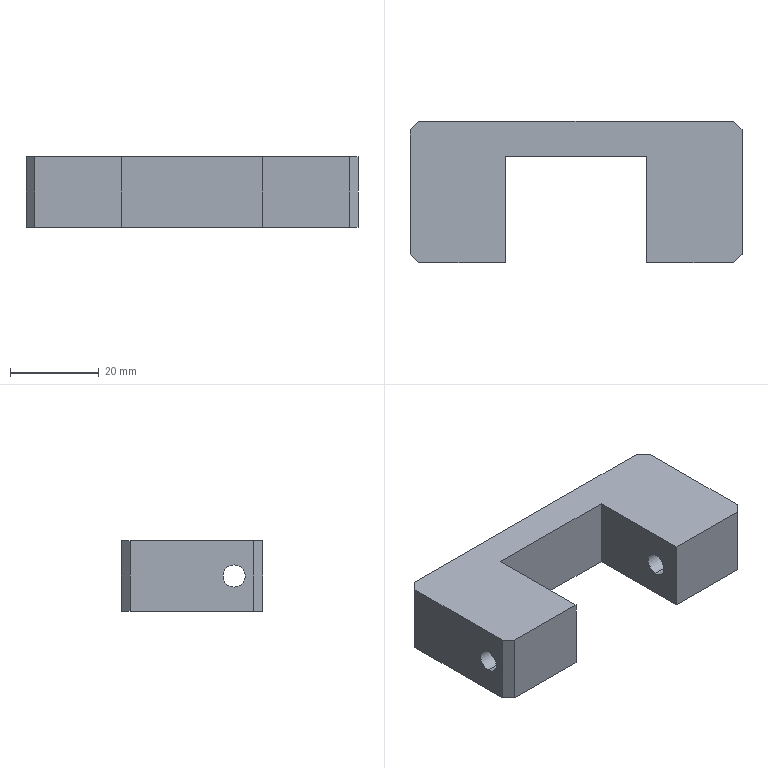Part | SolidWorks | features Chamfer 2, HoleWzd 2, Extrusion 1, ICE 1 | 1 solid | 26 faces | box 75 x 32 x 16 mm | volume 23656 mm3 | plane 14 | cylinder 8 | cone 4 | commonest cylinder face diameters 5 x4 6.8 x4
STEP:
#1=CARTESIAN_POINT('',(-27.5,-3.75,-3.4));
#2=VERTEX_POINT('',#1);
#3=CARTESIAN_POINT('',(-27.5,-3.75,3.4));
#4=VERTEX_POINT('',#3);
#5=CARTESIAN_POINT('',(-27.5,-3.75,0.));
#6=DIRECTION('',(0.,1.,0.));
#7=DIRECTION('',(0.,0.,1.));
#8=AXIS2_PLACEMENT_3D('',#5,#6,#7);
#9=CIRCLE('',#8,3.4);
#10=EDGE_CURVE('',#2,#4,#9,.T.);
#11=ORIENTED_EDGE('',*,*,#10,.F.);
#12=CARTESIAN_POINT('',(-27.5,16.,-3.4));
#13=VERTEX_POINT('',#12);
#14=CARTESIAN_POINT('',(-27.5,16.,-3.4));
#15=DIRECTION('',(0.,1.,0.));
#16=VECTOR('',#15,1000.);
#17=LINE('',#14,#16);
#18=EDGE_CURVE('',#2,#13,#17,.T.);
#19=ORIENTED_EDGE('',*,*,#18,.T.);
#20=CARTESIAN_POINT('',(-27.5,16.,3.4));
#21=VERTEX_POINT('',#20);
#22=CARTESIAN_POINT('',(-27.5,16.,0.));
#23=DIRECTION('',(0.,1.,0.));
#24=DIRECTION('',(0.,0.,1.));
#25=AXIS2_PLACEMENT_3D('',#22,#23,#24);
#26=CIRCLE('',#25,3.4);
#27=EDGE_CURVE('',#13,#21,#26,.T.);
#28=ORIENTED_EDGE('',*,*,#27,.T.);
#29=CARTESIAN_POINT('',(-27.5,16.,3.4));
#30=DIRECTION('',(0.,1.,0.));
#31=VECTOR('',#30,1000.);
#32=LINE('',#29,#31);
#33=EDGE_CURVE('',#4,#21,#32,.T.);
#34=ORIENTED_EDGE('',*,*,#33,.F.);
#35=EDGE_LOOP('',(#11,#19,#28,#34));
#36=FACE_OUTER_BOUND('',#35,.T.);
#37=CARTESIAN_POINT('',(-27.5,16.,0.));
#38=DIRECTION('',(0.,1.,0.));
#39=DIRECTION('',(0.,0.,1.));
#40=AXIS2_PLACEMENT_3D('',#37,#38,#39);
#41=CYLINDRICAL_SURFACE('',#40,3.4);
#42=ADVANCED_FACE('',(#36),#41,.F.);
#43=CARTESIAN_POINT('',(-27.5,-5.793,0.));
#44=VERTEX_POINT('',#43);
#45=CARTESIAN_POINT('',(-27.5,-3.75,3.4));
#46=DIRECTION('',(0.,0.515,0.8572));
#47=VECTOR('',#46,1000.);
#48=LINE('',#45,#47);
#49=EDGE_CURVE('',#44,#4,#48,.T.);
#50=ORIENTED_EDGE('',*,*,#49,.F.);
#51=CARTESIAN_POINT('',(-27.5,-3.75,-3.4));
#52=DIRECTION('',(0.,0.515,-0.8572));
#53=VECTOR('',#52,1000.);
#54=LINE('',#51,#53);
#55=EDGE_CURVE('',#44,#2,#54,.T.);
#56=ORIENTED_EDGE('',*,*,#55,.T.);
#57=ORIENTED_EDGE('',*,*,#10,.T.);
#58=EDGE_LOOP('',(#50,#56,#57));
#59=FACE_OUTER_BOUND('',#58,.T.);
#60=CARTESIAN_POINT('',(-27.5,-3.75,0.));
#61=DIRECTION('',(0.,1.,0.));
#62=DIRECTION('',(0.,0.,1.));
#63=AXIS2_PLACEMENT_3D('',#60,#61,#62);
#64=CONICAL_SURFACE('',#63,3.4,1.03);
#65=ADVANCED_FACE('',(#59),#64,.F.);
#66=CARTESIAN_POINT('',(27.5,-3.75,-3.4));
#67=VERTEX_POINT('',#66);
#68=CARTESIAN_POINT('',(27.5,-3.75,3.4));
#69=VERTEX_POINT('',#68);
#70=CARTESIAN_POINT('',(27.5,-3.75,0.));
#71=DIRECTION('',(0.,1.,0.));
#72=DIRECTION('',(0.,0.,1.));
#73=AXIS2_PLACEMENT_3D('',#70,#71,#72);
#74=CIRCLE('',#73,3.4);
#75=EDGE_CURVE('',#67,#69,#74,.T.);
#76=ORIENTED_EDGE('',*,*,#75,.F.);
#77=CARTESIAN_POINT('',(27.5,16.,-3.4));
#78=VERTEX_POINT('',#77);
#79=CARTESIAN_POINT('',(27.5,16.,-3.4));
#80=DIRECTION('',(0.,1.,0.));
#81=VECTOR('',#80,1000.);
#82=LINE('',#79,#81);
#83=EDGE_CURVE('',#67,#78,#82,.T.);
#84=ORIENTED_EDGE('',*,*,#83,.T.);
#85=CARTESIAN_POINT('',(27.5,16.,3.4));
#86=VERTEX_POINT('',#85);
#87=CARTESIAN_POINT('',(27.5,16.,0.));
#88=DIRECTION('',(0.,1.,0.));
#89=DIRECTION('',(0.,0.,1.));
#90=AXIS2_PLACEMENT_3D('',#87,#88,#89);
#91=CIRCLE('',#90,3.4);
#92=EDGE_CURVE('',#78,#86,#91,.T.);
#93=ORIENTED_EDGE('',*,*,#92,.T.);
#94=CARTESIAN_POINT('',(27.5,16.,3.4));
#95=DIRECTION('',(0.,1.,0.));
#96=VECTOR('',#95,1000.);
#97=LINE('',#94,#96);
#98=EDGE_CURVE('',#69,#86,#97,.T.);
#99=ORIENTED_EDGE('',*,*,#98,.F.);
#100=EDGE_LOOP('',(#76,#84,#93,#99));
#101=FACE_OUTER_BOUND('',#100,.T.);
#102=CARTESIAN_POINT('',(27.5,16.,0.));
#103=DIRECTION('',(0.,1.,0.));
#104=DIRECTION('',(0.,0.,1.));
#105=AXIS2_PLACEMENT_3D('',#102,#103,#104);
#106=CYLINDRICAL_SURFACE('',#105,3.4);
#107=ADVANCED_FACE('',(#101),#106,.F.);
#108=CARTESIAN_POINT('',(27.5,-5.793,0.));
#109=VERTEX_POINT('',#108);
#110=CARTESIAN_POINT('',(27.5,-3.75,3.4));
#111=DIRECTION('',(0.,0.515,0.8572));
#112=VECTOR('',#111,1000.);
#113=LINE('',#110,#112);
#114=EDGE_CURVE('',#109,#69,#113,.T.);
#115=ORIENTED_EDGE('',*,*,#114,.F.);
#116=CARTESIAN_POINT('',(27.5,-3.75,-3.4));
#117=DIRECTION('',(0.,0.515,-0.8572));
#118=VECTOR('',#117,1000.);
#119=LINE('',#116,#118);
#120=EDGE_CURVE('',#109,#67,#119,.T.);
#121=ORIENTED_EDGE('',*,*,#120,.T.);
#122=ORIENTED_EDGE('',*,*,#75,.T.);
#123=EDGE_LOOP('',(#115,#121,#122));
#124=FACE_OUTER_BOUND('',#123,.T.);
#125=CARTESIAN_POINT('',(27.5,-3.75,0.));
#126=DIRECTION('',(0.,1.,0.));
#127=DIRECTION('',(0.,0.,1.));
#128=AXIS2_PLACEMENT_3D('',#125,#126,#127);
#129=CONICAL_SURFACE('',#128,3.4,1.03);
#130=ADVANCED_FACE('',(#124),#129,.F.);
#131=CARTESIAN_POINT('',(-37.5,-9.5,2.5));
#132=VERTEX_POINT('',#131);
#133=CARTESIAN_POINT('',(-37.5,-9.5,-2.5));
#134=VERTEX_POINT('',#133);
#135=CARTESIAN_POINT('',(-37.5,-9.5,0.));
#136=DIRECTION('',(1.,0.,0.));
#137=DIRECTION('',(0.,0.,-1.));
#138=AXIS2_PLACEMENT_3D('',#135,#136,#137);
#139=CIRCLE('',#138,2.5);
#140=EDGE_CURVE('',#132,#134,#139,.T.);
#141=ORIENTED_EDGE('',*,*,#140,.F.);
#142=CARTESIAN_POINT('',(-16.,-9.5,2.5));
#143=VERTEX_POINT('',#142);
#144=CARTESIAN_POINT('',(37.5,-9.5,2.5));
#145=DIRECTION('',(1.,0.,0.));
#146=VECTOR('',#145,1000.);
#147=LINE('',#144,#146);
#148=EDGE_CURVE('',#132,#143,#147,.T.);
#149=ORIENTED_EDGE('',*,*,#148,.T.);
#150=CARTESIAN_POINT('',(-16.,-9.5,-2.5));
#151=VERTEX_POINT('',#150);
#152=CARTESIAN_POINT('',(-16.,-9.5,0.));
#153=DIRECTION('',(-1.,0.,0.));
#154=DIRECTION('',(0.,0.,1.));
#155=AXIS2_PLACEMENT_3D('',#152,#153,#154);
#156=CIRCLE('',#155,2.5);
#157=EDGE_CURVE('',#151,#143,#156,.T.);
#158=ORIENTED_EDGE('',*,*,#157,.F.);
#159=CARTESIAN_POINT('',(37.5,-9.5,-2.5));
#160=DIRECTION('',(1.,0.,0.));
#161=VECTOR('',#160,1000.);
#162=LINE('',#159,#161);
#163=EDGE_CURVE('',#134,#151,#162,.T.);
#164=ORIENTED_EDGE('',*,*,#163,.F.);
#165=EDGE_LOOP('',(#141,#149,#158,#164));
#166=FACE_OUTER_BOUND('',#165,.T.);
#167=CARTESIAN_POINT('',(37.5,-9.5,0.));
#168=DIRECTION('',(1.,0.,0.));
#169=DIRECTION('',(0.,0.,-1.));
#170=AXIS2_PLACEMENT_3D('',#167,#168,#169);
#171=CYLINDRICAL_SURFACE('',#170,2.5);
#172=ADVANCED_FACE('',(#166),#171,.F.);
#173=CARTESIAN_POINT('',(16.,-9.5,2.5));
#174=VERTEX_POINT('',#173);
#175=CARTESIAN_POINT('',(16.,-9.5,-2.5));
#176=VERTEX_POINT('',#175);
#177=CARTESIAN_POINT('',(16.,-9.5,0.));
#178=DIRECTION('',(1.,0.,0.));
#179=DIRECTION('',(0.,1.,0.));
#180=AXIS2_PLACEMENT_3D('',#177,#178,#179);
#181=CIRCLE('',#180,2.5);
#182=EDGE_CURVE('',#174,#176,#181,.T.);
#183=ORIENTED_EDGE('',*,*,#182,.F.);
#184=CARTESIAN_POINT('',(37.5,-9.5,2.5));
#185=VERTEX_POINT('',#184);
#186=CARTESIAN_POINT('',(37.5,-9.5,2.5));
#187=DIRECTION('',(1.,0.,0.));
#188=VECTOR('',#187,1000.);
#189=LINE('',#186,#188);
#190=EDGE_CURVE('',#174,#185,#189,.T.);
#191=ORIENTED_EDGE('',*,*,#190,.T.);
#192=CARTESIAN_POINT('',(37.5,-9.5,-2.5));
#193=VERTEX_POINT('',#192);
#194=CARTESIAN_POINT('',(37.5,-9.5,0.));
#195=DIRECTION('',(1.,0.,0.));
#196=DIRECTION('',(0.,0.,-1.));
#197=AXIS2_PLACEMENT_3D('',#194,#195,#196);
#198=CIRCLE('',#197,2.5);
#199=EDGE_CURVE('',#185,#193,#198,.T.);
#200=ORIENTED_EDGE('',*,*,#199,.T.);
#201=CARTESIAN_POINT('',(37.5,-9.5,-2.5));
#202=DIRECTION('',(1.,0.,0.));
#203=VECTOR('',#202,1000.);
#204=LINE('',#201,#203);
#205=EDGE_CURVE('',#176,#193,#204,.T.);
#206=ORIENTED_EDGE('',*,*,#205,.F.);
#207=EDGE_LOOP('',(#183,#191,#200,#206));
#208=FACE_OUTER_BOUND('',#207,.T.);
#209=CARTESIAN_POINT('',(37.5,-9.5,0.));
#210=DIRECTION('',(1.,0.,0.));
#211=DIRECTION('',(0.,0.,-1.));
#212=AXIS2_PLACEMENT_3D('',#209,#210,#211);
#213=CYLINDRICAL_SURFACE('',#212,2.5);
#214=ADVANCED_FACE('',(#208),#213,.F.);
#215=CARTESIAN_POINT('',(-35.5,-16.,8.));
#216=VERTEX_POINT('',#215);
#217=CARTESIAN_POINT('',(-16.,-16.,8.));
#218=VERTEX_POINT('',#217);
#219=CARTESIAN_POINT('',(-37.5,-16.,8.));
#220=DIRECTION('',(1.,0.,0.));
#221=VECTOR('',#220,1000.);
#222=LINE('',#219,#221);
#223=EDGE_CURVE('',#216,#218,#222,.T.);
#224=ORIENTED_EDGE('',*,*,#223,.F.);
#225=CARTESIAN_POINT('',(-35.5,-16.,-8.));
#226=VERTEX_POINT('',#225);
#227=CARTESIAN_POINT('',(-35.5,-16.,8.));
#228=DIRECTION('',(0.,0.,-1.));
#229=VECTOR('',#228,1000.);
#230=LINE('',#227,#229);
#231=EDGE_CURVE('',#216,#226,#230,.T.);
#232=ORIENTED_EDGE('',*,*,#231,.T.);
#233=CARTESIAN_POINT('',(-16.,-16.,-8.));
#234=VERTEX_POINT('',#233);
#235=CARTESIAN_POINT('',(-37.5,-16.,-8.));
#236=DIRECTION('',(1.,0.,0.));
#237=VECTOR('',#236,1000.);
#238=LINE('',#235,#237);
#239=EDGE_CURVE('',#226,#234,#238,.T.);
#240=ORIENTED_EDGE('',*,*,#239,.T.);
#241=CARTESIAN_POINT('',(-16.,-16.,-8.));
#242=DIRECTION('',(0.,0.,1.));
#243=VECTOR('',#242,1000.);
#244=LINE('',#241,#243);
#245=EDGE_CURVE('',#234,#218,#244,.T.);
#246=ORIENTED_EDGE('',*,*,#245,.T.);
#247=EDGE_LOOP('',(#224,#232,#240,#246));
#248=FACE_OUTER_BOUND('',#247,.T.);
#249=CARTESIAN_POINT('',(-37.5,-16.,8.));
#250=DIRECTION('',(0.,1.,0.));
#251=DIRECTION('',(0.,0.,1.));
#252=AXIS2_PLACEMENT_3D('',#249,#250,#251);
#253=PLANE('',#252);
#254=ADVANCED_FACE('',(#248),#253,.F.);
#255=CARTESIAN_POINT('',(-37.5,-9.5,0.));
#256=DIRECTION('',(1.,0.,0.));
#257=DIRECTION('',(0.,0.,-1.));
#258=AXIS2_PLACEMENT_3D('',#255,#256,#257);
#259=CIRCLE('',#258,2.5);
#260=EDGE_CURVE('',#134,#132,#259,.T.);
#261=ORIENTED_EDGE('',*,*,#260,.T.);
#262=ORIENTED_EDGE('',*,*,#140,.T.);
#263=EDGE_LOOP('',(#261,#262));
#264=FACE_BOUND('',#263,.T.);
#265=CARTESIAN_POINT('',(-37.5,14.,-8.));
#266=VERTEX_POINT('',#265);
#267=CARTESIAN_POINT('',(-37.5,-14.,-8.));
#268=VERTEX_POINT('',#267);
#269=CARTESIAN_POINT('',(-37.5,16.,-8.));
#270=DIRECTION('',(0.,-1.,0.));
#271=VECTOR('',#270,1000.);
#272=LINE('',#269,#271);
#273=EDGE_CURVE('',#266,#268,#272,.T.);
#274=ORIENTED_EDGE('',*,*,#273,.T.);
#275=CARTESIAN_POINT('',(-37.5,-14.,8.));
#276=VERTEX_POINT('',#275);
#277=CARTESIAN_POINT('',(-37.5,-14.,8.));
#278=DIRECTION('',(0.,0.,1.));
#279=VECTOR('',#278,1000.);
#280=LINE('',#277,#279);
#281=EDGE_CURVE('',#268,#276,#280,.T.);
#282=ORIENTED_EDGE('',*,*,#281,.T.);
#283=CARTESIAN_POINT('',(-37.5,14.,8.));
#284=VERTEX_POINT('',#283);
#285=CARTESIAN_POINT('',(-37.5,16.,8.));
#286=DIRECTION('',(0.,-1.,0.));
#287=VECTOR('',#286,1000.);
#288=LINE('',#285,#287);
#289=EDGE_CURVE('',#284,#276,#288,.T.);
#290=ORIENTED_EDGE('',*,*,#289,.F.);
#291=CARTESIAN_POINT('',(-37.5,14.,8.));
#292=DIRECTION('',(0.,0.,-1.));
#293=VECTOR('',#292,1000.);
#294=LINE('',#291,#293);
#295=EDGE_CURVE('',#284,#266,#294,.T.);
#296=ORIENTED_EDGE('',*,*,#295,.T.);
#297=EDGE_LOOP('',(#274,#282,#290,#296));
#298=FACE_OUTER_BOUND('',#297,.T.);
#299=CARTESIAN_POINT('',(-37.5,16.,8.));
#300=DIRECTION('',(1.,0.,0.));
#301=DIRECTION('',(0.,0.,-1.));
#302=AXIS2_PLACEMENT_3D('',#299,#300,#301);
#303=PLANE('',#302);
#304=ADVANCED_FACE('',(#264,#298),#303,.F.);
#305=CARTESIAN_POINT('',(16.,-16.,-8.));
#306=VERTEX_POINT('',#305);
#307=CARTESIAN_POINT('',(35.5,-16.,-8.));
#308=VERTEX_POINT('',#307);
#309=CARTESIAN_POINT('',(-37.5,-16.,-8.));
#310=DIRECTION('',(1.,0.,0.));
#311=VECTOR('',#310,1000.);
#312=LINE('',#309,#311);
#313=EDGE_CURVE('',#306,#308,#312,.T.);
#314=ORIENTED_EDGE('',*,*,#313,.T.);
#315=CARTESIAN_POINT('',(35.5,-16.,8.));
#316=VERTEX_POINT('',#315);
#317=CARTESIAN_POINT('',(35.5,-16.,8.));
#318=DIRECTION('',(0.,0.,1.));
#319=VECTOR('',#318,1000.);
#320=LINE('',#317,#319);
#321=EDGE_CURVE('',#308,#316,#320,.T.);
#322=ORIENTED_EDGE('',*,*,#321,.T.);
#323=CARTESIAN_POINT('',(16.,-16.,8.));
#324=VERTEX_POINT('',#323);
#325=CARTESIAN_POINT('',(-37.5,-16.,8.));
#326=DIRECTION('',(1.,0.,0.));
#327=VECTOR('',#326,1000.);
#328=LINE('',#325,#327);
#329=EDGE_CURVE('',#324,#316,#328,.T.);
#330=ORIENTED_EDGE('',*,*,#329,.F.);
#331=CARTESIAN_POINT('',(16.,-16.,-8.));
#332=DIRECTION('',(0.,0.,1.));
#333=VECTOR('',#332,1000.);
#334=LINE('',#331,#333);
#335=EDGE_CURVE('',#306,#324,#334,.T.);
#336=ORIENTED_EDGE('',*,*,#335,.F.);
#337=EDGE_LOOP('',(#314,#322,#330,#336));
#338=FACE_OUTER_BOUND('',#337,.T.);
#339=CARTESIAN_POINT('',(-37.5,-16.,8.));
#340=DIRECTION('',(0.,1.,0.));
#341=DIRECTION('',(0.,0.,1.));
#342=AXIS2_PLACEMENT_3D('',#339,#340,#341);
#343=PLANE('',#342);
#344=ADVANCED_FACE('',(#338),#343,.F.);
#345=CARTESIAN_POINT('',(37.5,-9.5,0.));
#346=DIRECTION('',(1.,0.,0.));
#347=DIRECTION('',(0.,0.,-1.));
#348=AXIS2_PLACEMENT_3D('',#345,#346,#347);
#349=CIRCLE('',#348,2.5);
#350=EDGE_CURVE('',#193,#185,#349,.T.);
#351=ORIENTED_EDGE('',*,*,#350,.F.);
#352=ORIENTED_EDGE('',*,*,#199,.F.);
#353=EDGE_LOOP('',(#351,#352));
#354=FACE_BOUND('',#353,.T.);
#355=CARTESIAN_POINT('',(37.5,-14.,8.));
#356=VERTEX_POINT('',#355);
#357=CARTESIAN_POINT('',(37.5,14.,8.));
#358=VERTEX_POINT('',#357);
#359=CARTESIAN_POINT('',(37.5,16.,8.));
#360=DIRECTION('',(0.,1.,0.));
#361=VECTOR('',#360,1000.);
#362=LINE('',#359,#361);
#363=EDGE_CURVE('',#356,#358,#362,.T.);
#364=ORIENTED_EDGE('',*,*,#363,.F.);
#365=CARTESIAN_POINT('',(37.5,-14.,-8.));
#366=VERTEX_POINT('',#365);
#367=CARTESIAN_POINT('',(37.5,-14.,8.));
#368=DIRECTION('',(0.,0.,-1.));
#369=VECTOR('',#368,1000.);
#370=LINE('',#367,#369);
#371=EDGE_CURVE('',#356,#366,#370,.T.);
#372=ORIENTED_EDGE('',*,*,#371,.T.);
#373=CARTESIAN_POINT('',(37.5,14.,-8.));
#374=VERTEX_POINT('',#373);
#375=CARTESIAN_POINT('',(37.5,16.,-8.));
#376=DIRECTION('',(0.,1.,0.));
#377=VECTOR('',#376,1000.);
#378=LINE('',#375,#377);
#379=EDGE_CURVE('',#366,#374,#378,.T.);
#380=ORIENTED_EDGE('',*,*,#379,.T.);
#381=CARTESIAN_POINT('',(37.5,14.,8.));
#382=DIRECTION('',(0.,0.,1.));
#383=VECTOR('',#382,1000.);
#384=LINE('',#381,#383);
#385=EDGE_CURVE('',#374,#358,#384,.T.);
#386=ORIENTED_EDGE('',*,*,#385,.T.);
#387=EDGE_LOOP('',(#364,#372,#380,#386));
#388=FACE_OUTER_BOUND('',#387,.T.);
#389=CARTESIAN_POINT('',(37.5,16.,8.));
#390=DIRECTION('',(-1.,0.,0.));
#391=DIRECTION('',(0.,0.,1.));
#392=AXIS2_PLACEMENT_3D('',#389,#390,#391);
#393=PLANE('',#392);
#394=ADVANCED_FACE('',(#354,#388),#393,.F.);
#395=CARTESIAN_POINT('',(-27.5,16.,0.));
#396=DIRECTION('',(0.,1.,0.));
#397=DIRECTION('',(0.,0.,1.));
#398=AXIS2_PLACEMENT_3D('',#395,#396,#397);
#399=CIRCLE('',#398,3.4);
#400=EDGE_CURVE('',#21,#13,#399,.T.);
#401=ORIENTED_EDGE('',*,*,#400,.F.);
#402=ORIENTED_EDGE('',*,*,#27,.F.);
#403=EDGE_LOOP('',(#401,#402));
#404=FACE_BOUND('',#403,.T.);
#405=CARTESIAN_POINT('',(27.5,16.,0.));
#406=DIRECTION('',(0.,1.,0.));
#407=DIRECTION('',(0.,0.,1.));
#408=AXIS2_PLACEMENT_3D('',#405,#406,#407);
#409=CIRCLE('',#408,3.4);
#410=EDGE_CURVE('',#86,#78,#409,.T.);
#411=ORIENTED_EDGE('',*,*,#410,.F.);
#412=ORIENTED_EDGE('',*,*,#92,.F.);
#413=EDGE_LOOP('',(#411,#412));
#414=FACE_BOUND('',#413,.T.);
#415=CARTESIAN_POINT('',(35.5,16.,-8.));
#416=VERTEX_POINT('',#415);
#417=CARTESIAN_POINT('',(-35.5,16.,-8.));
#418=VERTEX_POINT('',#417);
#419=CARTESIAN_POINT('',(-37.5,16.,-8.));
#420=DIRECTION('',(-1.,0.,0.));
#421=VECTOR('',#420,1000.);
#422=LINE('',#419,#421);
#423=EDGE_CURVE('',#416,#418,#422,.T.);
#424=ORIENTED_EDGE('',*,*,#423,.T.);
#425=CARTESIAN_POINT('',(-35.5,16.,8.));
#426=VERTEX_POINT('',#425);
#427=CARTESIAN_POINT('',(-35.5,16.,8.));
#428=DIRECTION('',(0.,0.,1.));
#429=VECTOR('',#428,1000.);
#430=LINE('',#427,#429);
#431=EDGE_CURVE('',#418,#426,#430,.T.);
#432=ORIENTED_EDGE('',*,*,#431,.T.);
#433=CARTESIAN_POINT('',(35.5,16.,8.));
#434=VERTEX_POINT('',#433);
#435=CARTESIAN_POINT('',(-37.5,16.,8.));
#436=DIRECTION('',(-1.,0.,0.));
#437=VECTOR('',#436,1000.);
#438=LINE('',#435,#437);
#439=EDGE_CURVE('',#434,#426,#438,.T.);
#440=ORIENTED_EDGE('',*,*,#439,.F.);
#441=CARTESIAN_POINT('',(35.5,16.,8.));
#442=DIRECTION('',(0.,0.,-1.));
#443=VECTOR('',#442,1000.);
#444=LINE('',#441,#443);
#445=EDGE_CURVE('',#434,#416,#444,.T.);
#446=ORIENTED_EDGE('',*,*,#445,.T.);
#447=EDGE_LOOP('',(#424,#432,#440,#446));
#448=FACE_OUTER_BOUND('',#447,.T.);
#449=CARTESIAN_POINT('',(-37.5,16.,8.));
#450=DIRECTION('',(0.,-1.,0.));
#451=DIRECTION('',(0.,0.,-1.));
#452=AXIS2_PLACEMENT_3D('',#449,#450,#451);
#453=PLANE('',#452);
#454=ADVANCED_FACE('',(#404,#414,#448),#453,.F.);
#455=ORIENTED_EDGE('',*,*,#329,.T.);
#456=CARTESIAN_POINT('',(25.75,-25.75,8.));
#457=DIRECTION('',(0.7071,0.7071,0.));
#458=VECTOR('',#457,1000.);
#459=LINE('',#456,#458);
#460=EDGE_CURVE('',#316,#356,#459,.T.);
#461=ORIENTED_EDGE('',*,*,#460,.T.);
#462=ORIENTED_EDGE('',*,*,#363,.T.);
#463=CARTESIAN_POINT('',(25.75,25.75,8.));
#464=DIRECTION('',(-0.7071,0.7071,0.));
#465=VECTOR('',#464,1000.);
#466=LINE('',#463,#465);
#467=EDGE_CURVE('',#358,#434,#466,.T.);
#468=ORIENTED_EDGE('',*,*,#467,.T.);
#469=ORIENTED_EDGE('',*,*,#439,.T.);
#470=CARTESIAN_POINT('',(-25.75,25.75,8.));
#471=DIRECTION('',(-0.7071,-0.7071,0.));
#472=VECTOR('',#471,1000.);
#473=LINE('',#470,#472);
#474=EDGE_CURVE('',#426,#284,#473,.T.);
#475=ORIENTED_EDGE('',*,*,#474,.T.);
#476=ORIENTED_EDGE('',*,*,#289,.T.);
#477=CARTESIAN_POINT('',(-25.75,-25.75,8.));
#478=DIRECTION('',(0.7071,-0.7071,0.));
#479=VECTOR('',#478,1000.);
#480=LINE('',#477,#479);
#481=EDGE_CURVE('',#276,#216,#480,.T.);
#482=ORIENTED_EDGE('',*,*,#481,.T.);
#483=ORIENTED_EDGE('',*,*,#223,.T.);
#484=CARTESIAN_POINT('',(-16.,8.,8.));
#485=VERTEX_POINT('',#484);
#486=CARTESIAN_POINT('',(-16.,-16.,8.));
#487=DIRECTION('',(0.,-1.,0.));
#488=VECTOR('',#487,1000.);
#489=LINE('',#486,#488);
#490=EDGE_CURVE('',#485,#218,#489,.T.);
#491=ORIENTED_EDGE('',*,*,#490,.F.);
#492=CARTESIAN_POINT('',(16.,8.,8.));
#493=VERTEX_POINT('',#492);
#494=CARTESIAN_POINT('',(-16.,8.,8.));
#495=DIRECTION('',(-1.,0.,0.));
#496=VECTOR('',#495,1000.);
#497=LINE('',#494,#496);
#498=EDGE_CURVE('',#493,#485,#497,.T.);
#499=ORIENTED_EDGE('',*,*,#498,.F.);
#500=CARTESIAN_POINT('',(16.,-16.,8.));
#501=DIRECTION('',(0.,1.,0.));
#502=VECTOR('',#501,1000.);
#503=LINE('',#500,#502);
#504=EDGE_CURVE('',#324,#493,#503,.T.);
#505=ORIENTED_EDGE('',*,*,#504,.F.);
#506=EDGE_LOOP('',(#455,#461,#462,#468,#469,#475,#476,#482,#483,#491,#499,#505));
#507=FACE_OUTER_BOUND('',#506,.T.);
#508=CARTESIAN_POINT('',(0.,0.,8.));
#509=DIRECTION('',(0.,0.,1.));
#510=DIRECTION('',(1.,0.,0.));
#511=AXIS2_PLACEMENT_3D('',#508,#509,#510);
#512=PLANE('',#511);
#513=ADVANCED_FACE('',(#507),#512,.T.);
#514=ORIENTED_EDGE('',*,*,#379,.F.);
#515=CARTESIAN_POINT('',(37.5,-14.,-8.));
#516=DIRECTION('',(-0.7071,-0.7071,0.));
#517=VECTOR('',#516,1000.);
#518=LINE('',#515,#517);
#519=EDGE_CURVE('',#366,#308,#518,.T.);
#520=ORIENTED_EDGE('',*,*,#519,.T.);
#521=ORIENTED_EDGE('',*,*,#313,.F.);
#522=CARTESIAN_POINT('',(16.,8.,-8.));
#523=VERTEX_POINT('',#522);
#524=CARTESIAN_POINT('',(16.,-16.,-8.));
#525=DIRECTION('',(0.,1.,0.));
#526=VECTOR('',#525,1000.);
#527=LINE('',#524,#526);
#528=EDGE_CURVE('',#306,#523,#527,.T.);
#529=ORIENTED_EDGE('',*,*,#528,.T.);
#530=CARTESIAN_POINT('',(-16.,8.,-8.));
#531=VERTEX_POINT('',#530);
#532=CARTESIAN_POINT('',(-16.,8.,-8.));
#533=DIRECTION('',(-1.,0.,0.));
#534=VECTOR('',#533,1000.);
#535=LINE('',#532,#534);
#536=EDGE_CURVE('',#523,#531,#535,.T.);
#537=ORIENTED_EDGE('',*,*,#536,.T.);
#538=CARTESIAN_POINT('',(-16.,-16.,-8.));
#539=DIRECTION('',(0.,-1.,0.));
#540=VECTOR('',#539,1000.);
#541=LINE('',#538,#540);
#542=EDGE_CURVE('',#531,#234,#541,.T.);
#543=ORIENTED_EDGE('',*,*,#542,.T.);
#544=ORIENTED_EDGE('',*,*,#239,.F.);
#545=CARTESIAN_POINT('',(-35.5,-16.,-8.));
#546=DIRECTION('',(-0.7071,0.7071,0.));
#547=VECTOR('',#546,1000.);
#548=LINE('',#545,#547);
#549=EDGE_CURVE('',#226,#268,#548,.T.);
#550=ORIENTED_EDGE('',*,*,#549,.T.);
#551=ORIENTED_EDGE('',*,*,#273,.F.);
#552=CARTESIAN_POINT('',(-37.5,14.,-8.));
#553=DIRECTION('',(0.7071,0.7071,0.));
#554=VECTOR('',#553,1000.);
#555=LINE('',#552,#554);
#556=EDGE_CURVE('',#266,#418,#555,.T.);
#557=ORIENTED_EDGE('',*,*,#556,.T.);
#558=ORIENTED_EDGE('',*,*,#423,.F.);
#559=CARTESIAN_POINT('',(35.5,16.,-8.));
#560=DIRECTION('',(0.7071,-0.7071,0.));
#561=VECTOR('',#560,1000.);
#562=LINE('',#559,#561);
#563=EDGE_CURVE('',#416,#374,#562,.T.);
#564=ORIENTED_EDGE('',*,*,#563,.T.);
#565=EDGE_LOOP('',(#514,#520,#521,#529,#537,#543,#544,#550,#551,#557,#558,#564));
#566=FACE_OUTER_BOUND('',#565,.T.);
#567=CARTESIAN_POINT('',(0.,0.,-8.));
#568=DIRECTION('',(0.,0.,1.));
#569=DIRECTION('',(1.,0.,0.));
#570=AXIS2_PLACEMENT_3D('',#567,#568,#569);
#571=PLANE('',#570);
#572=ADVANCED_FACE('',(#566),#571,.F.);
#573=ORIENTED_EDGE('',*,*,#157,.T.);
#574=CARTESIAN_POINT('',(-16.,-9.5,0.));
#575=DIRECTION('',(-1.,0.,0.));
#576=DIRECTION('',(0.,0.,1.));
#577=AXIS2_PLACEMENT_3D('',#574,#575,#576);
#578=CIRCLE('',#577,2.5);
#579=EDGE_CURVE('',#143,#151,#578,.T.);
#580=ORIENTED_EDGE('',*,*,#579,.T.);
#581=EDGE_LOOP('',(#573,#580));
#582=FACE_BOUND('',#581,.T.);
#583=ORIENTED_EDGE('',*,*,#490,.T.);
#584=ORIENTED_EDGE('',*,*,#245,.F.);
#585=ORIENTED_EDGE('',*,*,#542,.F.);
#586=CARTESIAN_POINT('',(-16.,8.,-8.));
#587=DIRECTION('',(0.,0.,1.));
#588=VECTOR('',#587,1000.);
#589=LINE('',#586,#588);
#590=EDGE_CURVE('',#531,#485,#589,.T.);
#591=ORIENTED_EDGE('',*,*,#590,.T.);
#592=EDGE_LOOP('',(#583,#584,#585,#591));
#593=FACE_OUTER_BOUND('',#592,.T.);
#594=CARTESIAN_POINT('',(-16.,-16.,-8.));
#595=DIRECTION('',(-1.,0.,0.));
#596=DIRECTION('',(0.,0.,1.));
#597=AXIS2_PLACEMENT_3D('',#594,#595,#596);
#598=PLANE('',#597);
#599=ADVANCED_FACE('',(#582,#593),#598,.F.);
#600=ORIENTED_EDGE('',*,*,#498,.T.);
#601=ORIENTED_EDGE('',*,*,#590,.F.);
#602=ORIENTED_EDGE('',*,*,#536,.F.);
#603=CARTESIAN_POINT('',(16.,8.,-8.));
#604=DIRECTION('',(0.,0.,1.));
#605=VECTOR('',#604,1000.);
#606=LINE('',#603,#605);
#607=EDGE_CURVE('',#523,#493,#606,.T.);
#608=ORIENTED_EDGE('',*,*,#607,.T.);
#609=EDGE_LOOP('',(#600,#601,#602,#608));
#610=FACE_OUTER_BOUND('',#609,.T.);
#611=CARTESIAN_POINT('',(-16.,8.,-8.));
#612=DIRECTION('',(0.,1.,0.));
#613=DIRECTION('',(-1.,0.,0.));
#614=AXIS2_PLACEMENT_3D('',#611,#612,#613);
#615=PLANE('',#614);
#616=ADVANCED_FACE('',(#610),#615,.F.);
#617=CARTESIAN_POINT('',(16.,-9.5,0.));
#618=DIRECTION('',(1.,0.,0.));
#619=DIRECTION('',(0.,1.,0.));
#620=AXIS2_PLACEMENT_3D('',#617,#618,#619);
#621=CIRCLE('',#620,2.5);
#622=EDGE_CURVE('',#176,#174,#621,.T.);
#623=ORIENTED_EDGE('',*,*,#622,.T.);
#624=ORIENTED_EDGE('',*,*,#182,.T.);
#625=EDGE_LOOP('',(#623,#624));
#626=FACE_BOUND('',#625,.T.);
#627=ORIENTED_EDGE('',*,*,#504,.T.);
#628=ORIENTED_EDGE('',*,*,#607,.F.);
#629=ORIENTED_EDGE('',*,*,#528,.F.);
#630=ORIENTED_EDGE('',*,*,#335,.T.);
#631=EDGE_LOOP('',(#627,#628,#629,#630));
#632=FACE_OUTER_BOUND('',#631,.T.);
#633=CARTESIAN_POINT('',(16.,-16.,-8.));
#634=DIRECTION('',(1.,0.,0.));
#635=DIRECTION('',(0.,1.,0.));
#636=AXIS2_PLACEMENT_3D('',#633,#634,#635);
#637=PLANE('',#636);
#638=ADVANCED_FACE('',(#626,#632),#637,.F.);
#639=ORIENTED_EDGE('',*,*,#190,.F.);
#640=ORIENTED_EDGE('',*,*,#622,.F.);
#641=ORIENTED_EDGE('',*,*,#205,.T.);
#642=ORIENTED_EDGE('',*,*,#350,.T.);
#643=EDGE_LOOP('',(#639,#640,#641,#642));
#644=FACE_OUTER_BOUND('',#643,.T.);
#645=CARTESIAN_POINT('',(37.5,-9.5,0.));
#646=DIRECTION('',(1.,0.,0.));
#647=DIRECTION('',(0.,0.,-1.));
#648=AXIS2_PLACEMENT_3D('',#645,#646,#647);
#649=CYLINDRICAL_SURFACE('',#648,2.5);
#650=ADVANCED_FACE('',(#644),#649,.F.);
#651=ORIENTED_EDGE('',*,*,#148,.F.);
#652=ORIENTED_EDGE('',*,*,#260,.F.);
#653=ORIENTED_EDGE('',*,*,#163,.T.);
#654=ORIENTED_EDGE('',*,*,#579,.F.);
#655=EDGE_LOOP('',(#651,#652,#653,#654));
#656=FACE_OUTER_BOUND('',#655,.T.);
#657=CARTESIAN_POINT('',(37.5,-9.5,0.));
#658=DIRECTION('',(1.,0.,0.));
#659=DIRECTION('',(0.,0.,-1.));
#660=AXIS2_PLACEMENT_3D('',#657,#658,#659);
#661=CYLINDRICAL_SURFACE('',#660,2.5);
#662=ADVANCED_FACE('',(#656),#661,.F.);
#663=ORIENTED_EDGE('',*,*,#474,.F.);
#664=ORIENTED_EDGE('',*,*,#431,.F.);
#665=ORIENTED_EDGE('',*,*,#556,.F.);
#666=ORIENTED_EDGE('',*,*,#295,.F.);
#667=EDGE_LOOP('',(#663,#664,#665,#666));
#668=FACE_OUTER_BOUND('',#667,.T.);
#669=CARTESIAN_POINT('',(-37.5,14.,8.));
#670=DIRECTION('',(0.7071,-0.7071,0.));
#671=DIRECTION('',(0.,0.,-1.));
#672=AXIS2_PLACEMENT_3D('',#669,#670,#671);
#673=PLANE('',#672);
#674=ADVANCED_FACE('',(#668),#673,.F.);
#675=ORIENTED_EDGE('',*,*,#467,.F.);
#676=ORIENTED_EDGE('',*,*,#385,.F.);
#677=ORIENTED_EDGE('',*,*,#563,.F.);
#678=ORIENTED_EDGE('',*,*,#445,.F.);
#679=EDGE_LOOP('',(#675,#676,#677,#678));
#680=FACE_OUTER_BOUND('',#679,.T.);
#681=CARTESIAN_POINT('',(35.5,16.,8.));
#682=DIRECTION('',(-0.7071,-0.7071,0.));
#683=DIRECTION('',(0.,0.,-1.));
#684=AXIS2_PLACEMENT_3D('',#681,#682,#683);
#685=PLANE('',#684);
#686=ADVANCED_FACE('',(#680),#685,.F.);
#687=ORIENTED_EDGE('',*,*,#120,.F.);
#688=ORIENTED_EDGE('',*,*,#114,.T.);
#689=CARTESIAN_POINT('',(27.5,-3.75,0.));
#690=DIRECTION('',(0.,1.,0.));
#691=DIRECTION('',(0.,0.,1.));
#692=AXIS2_PLACEMENT_3D('',#689,#690,#691);
#693=CIRCLE('',#692,3.4);
#694=EDGE_CURVE('',#69,#67,#693,.T.);
#695=ORIENTED_EDGE('',*,*,#694,.T.);
#696=EDGE_LOOP('',(#687,#688,#695));
#697=FACE_OUTER_BOUND('',#696,.T.);
#698=CARTESIAN_POINT('',(27.5,-3.75,0.));
#699=DIRECTION('',(0.,1.,0.));
#700=DIRECTION('',(0.,0.,1.));
#701=AXIS2_PLACEMENT_3D('',#698,#699,#700);
#702=CONICAL_SURFACE('',#701,3.4,1.03);
#703=ADVANCED_FACE('',(#697),#702,.F.);
#704=ORIENTED_EDGE('',*,*,#83,.F.);
#705=ORIENTED_EDGE('',*,*,#694,.F.);
#706=ORIENTED_EDGE('',*,*,#98,.T.);
#707=ORIENTED_EDGE('',*,*,#410,.T.);
#708=EDGE_LOOP('',(#704,#705,#706,#707));
#709=FACE_OUTER_BOUND('',#708,.T.);
#710=CARTESIAN_POINT('',(27.5,16.,0.));
#711=DIRECTION('',(0.,1.,0.));
#712=DIRECTION('',(0.,0.,1.));
#713=AXIS2_PLACEMENT_3D('',#710,#711,#712);
#714=CYLINDRICAL_SURFACE('',#713,3.4);
#715=ADVANCED_FACE('',(#709),#714,.F.);
#716=ORIENTED_EDGE('',*,*,#55,.F.);
#717=ORIENTED_EDGE('',*,*,#49,.T.);
#718=CARTESIAN_POINT('',(-27.5,-3.75,0.));
#719=DIRECTION('',(0.,1.,0.));
#720=DIRECTION('',(0.,0.,1.));
#721=AXIS2_PLACEMENT_3D('',#718,#719,#720);
#722=CIRCLE('',#721,3.4);
#723=EDGE_CURVE('',#4,#2,#722,.T.);
#724=ORIENTED_EDGE('',*,*,#723,.T.);
#725=EDGE_LOOP('',(#716,#717,#724));
#726=FACE_OUTER_BOUND('',#725,.T.);
#727=CARTESIAN_POINT('',(-27.5,-3.75,0.));
#728=DIRECTION('',(0.,1.,0.));
#729=DIRECTION('',(0.,0.,1.));
#730=AXIS2_PLACEMENT_3D('',#727,#728,#729);
#731=CONICAL_SURFACE('',#730,3.4,1.03);
#732=ADVANCED_FACE('',(#726),#731,.F.);
#733=ORIENTED_EDGE('',*,*,#18,.F.);
#734=ORIENTED_EDGE('',*,*,#723,.F.);
#735=ORIENTED_EDGE('',*,*,#33,.T.);
#736=ORIENTED_EDGE('',*,*,#400,.T.);
#737=EDGE_LOOP('',(#733,#734,#735,#736));
#738=FACE_OUTER_BOUND('',#737,.T.);
#739=CARTESIAN_POINT('',(-27.5,16.,0.));
#740=DIRECTION('',(0.,1.,0.));
#741=DIRECTION('',(0.,0.,1.));
#742=AXIS2_PLACEMENT_3D('',#739,#740,#741);
#743=CYLINDRICAL_SURFACE('',#742,3.4);
#744=ADVANCED_FACE('',(#738),#743,.F.);
#745=ORIENTED_EDGE('',*,*,#460,.F.);
#746=ORIENTED_EDGE('',*,*,#321,.F.);
#747=ORIENTED_EDGE('',*,*,#519,.F.);
#748=ORIENTED_EDGE('',*,*,#371,.F.);
#749=EDGE_LOOP('',(#745,#746,#747,#748));
#750=FACE_OUTER_BOUND('',#749,.T.);
#751=CARTESIAN_POINT('',(37.5,-14.,8.));
#752=DIRECTION('',(-0.7071,0.7071,0.));
#753=DIRECTION('',(0.,0.,-1.));
#754=AXIS2_PLACEMENT_3D('',#751,#752,#753);
#755=PLANE('',#754);
#756=ADVANCED_FACE('',(#750),#755,.F.);
#757=ORIENTED_EDGE('',*,*,#481,.F.);
#758=ORIENTED_EDGE('',*,*,#281,.F.);
#759=ORIENTED_EDGE('',*,*,#549,.F.);
#760=ORIENTED_EDGE('',*,*,#231,.F.);
#761=EDGE_LOOP('',(#757,#758,#759,#760));
#762=FACE_OUTER_BOUND('',#761,.T.);
#763=CARTESIAN_POINT('',(-35.5,-16.,8.));
#764=DIRECTION('',(0.7071,0.7071,0.));
#765=DIRECTION('',(0.,0.,-1.));
#766=AXIS2_PLACEMENT_3D('',#763,#764,#765);
#767=PLANE('',#766);
#768=ADVANCED_FACE('',(#762),#767,.F.);
#769=CLOSED_SHELL('',(#42,#65,#107,#130,#172,#214,#254,#304,#344,#394,#454,#513,#572,#599,#616,#638,#650,#662,#674,#686,#703,#715,#732,#744,#756,#768));
#770=MANIFOLD_SOLID_BREP('',#769);
#771=CARTESIAN_POINT('',(0.,0.,0.));
#772=DIRECTION('',(0.,0.,1.));
#773=DIRECTION('',(1.,0.,0.));
#774=AXIS2_PLACEMENT_3D('',#771,#772,#773);
#775=(LENGTH_UNIT()NAMED_UNIT(*)SI_UNIT(.MILLI.,.METRE.));
#776=UNCERTAINTY_MEASURE_WITH_UNIT(LENGTH_MEASURE(0.00001),#775,'','');
#777=(NAMED_UNIT(*)PLANE_ANGLE_UNIT()SI_UNIT($,.RADIAN.));
#778=(NAMED_UNIT(*)SI_UNIT($,.STERADIAN.)SOLID_ANGLE_UNIT());
#779=(GEOMETRIC_REPRESENTATION_CONTEXT(3)GLOBAL_UNCERTAINTY_ASSIGNED_CONTEXT((#776))GLOBAL_UNIT_ASSIGNED_CONTEXT((#775,#777,#778))REPRESENTATION_CONTEXT('',''));
#780=ADVANCED_BREP_SHAPE_REPRESENTATION('',(#770,#774),#779);